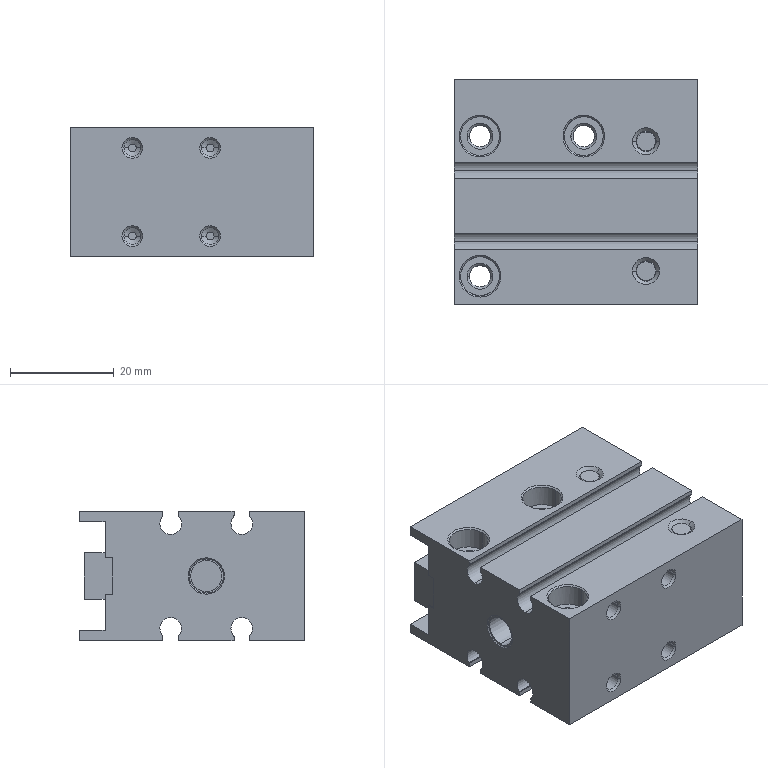Part | SolidWorks | features BaseBody 1 | 1 solid | 203 faces | box 47 x 43.5 x 25 mm | volume 36569 mm3 | cone 84 | cylinder 60 | plane 59 | commonest cylinder face diameters 3.242 x16 7.5 x12 4.134 x10 0.4 x8 4.2 x6 6 x2